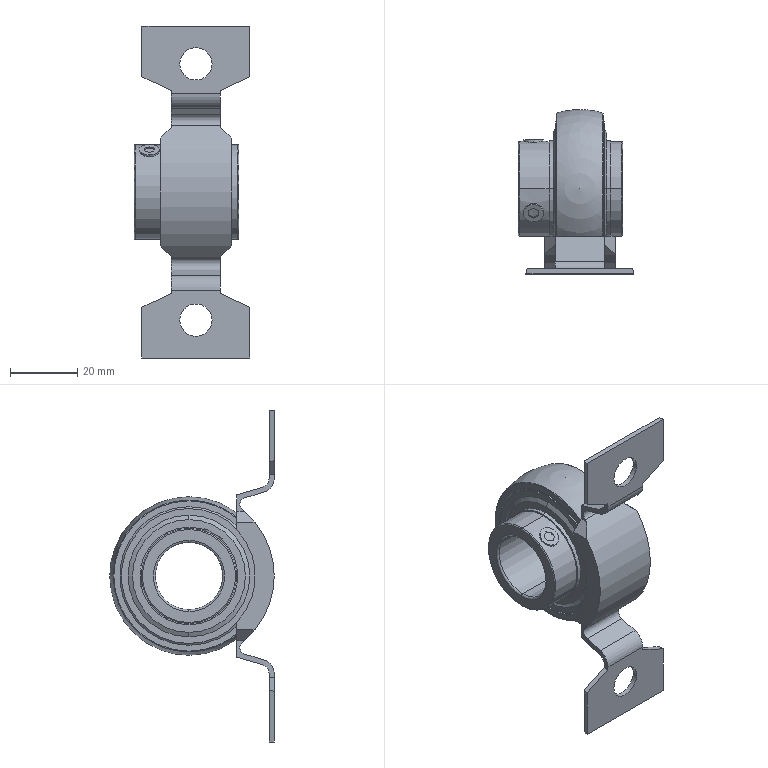Part | SolidWorks | features AEMSimFeature 1 | 10 solids | 249 faces | box 34.3 x 48.8 x 98.5 mm | volume 23790 mm3 | plane 72 | cone 62 | cylinder 59 | torus 36 | sphere 20 | commonest cylinder face diameters 28.2 x14 6 x6 9.6 x4 28.994 x4 29.008 x4 29.391 x4